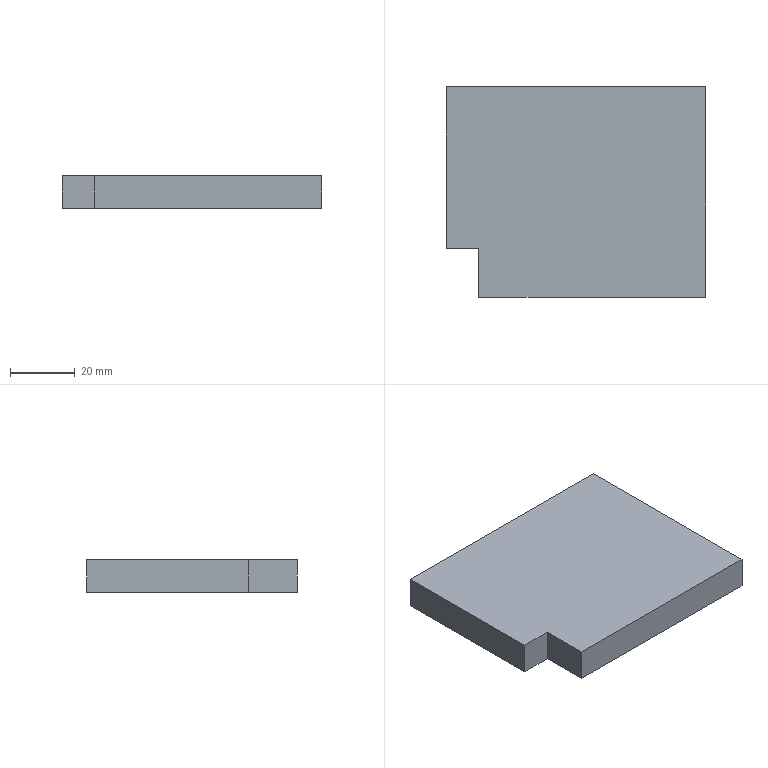Part | NX | features solid 2 | 1 solid | 8 faces | box 80 x 65 x 10 mm | volume 50500 mm3 | plane 8
STEP:
#1=CARTESIAN_POINT('',(-320.,0.,10.));
#2=VERTEX_POINT('',#1);
#3=CARTESIAN_POINT('',(-320.,0.,0.));
#4=VERTEX_POINT('',#3);
#5=CARTESIAN_POINT('',(-320.,0.,0.));
#6=DIRECTION('',(0.,0.,-1.));
#7=VECTOR('',#6,1000.);
#8=LINE('',#5,#7);
#9=EDGE_CURVE('',#2,#4,#8,.T.);
#10=ORIENTED_EDGE('',*,*,#9,.T.);
#11=CARTESIAN_POINT('',(-320.,-15.,0.));
#12=VERTEX_POINT('',#11);
#13=CARTESIAN_POINT('',(-320.,50.,0.));
#14=DIRECTION('',(0.,1.,0.));
#15=VECTOR('',#14,1000.);
#16=LINE('',#13,#15);
#17=EDGE_CURVE('',#12,#4,#16,.T.);
#18=ORIENTED_EDGE('',*,*,#17,.F.);
#19=CARTESIAN_POINT('',(-320.,-15.,10.));
#20=VERTEX_POINT('',#19);
#21=CARTESIAN_POINT('',(-320.,-15.,0.));
#22=DIRECTION('',(0.,0.,-1.));
#23=VECTOR('',#22,1000.);
#24=LINE('',#21,#23);
#25=EDGE_CURVE('',#20,#12,#24,.T.);
#26=ORIENTED_EDGE('',*,*,#25,.F.);
#27=CARTESIAN_POINT('',(-320.,50.,10.));
#28=DIRECTION('',(0.,1.,0.));
#29=VECTOR('',#28,1000.);
#30=LINE('',#27,#29);
#31=EDGE_CURVE('',#20,#2,#30,.T.);
#32=ORIENTED_EDGE('',*,*,#31,.T.);
#33=EDGE_LOOP('',(#10,#18,#26,#32));
#34=FACE_BOUND('',#33,.T.);
#35=CARTESIAN_POINT('',(-320.,50.,0.));
#36=DIRECTION('',(1.,0.,0.));
#37=DIRECTION('',(0.,-1.,0.));
#38=AXIS2_PLACEMENT_3D('',#35,#36,#37);
#39=PLANE('',#38);
#40=ADVANCED_FACE('',(#34),#39,.F.);
#41=CARTESIAN_POINT('',(-330.,0.,10.));
#42=VERTEX_POINT('',#41);
#43=CARTESIAN_POINT('',(-330.,0.,0.));
#44=VERTEX_POINT('',#43);
#45=CARTESIAN_POINT('',(-330.,0.,0.));
#46=DIRECTION('',(0.,0.,-1.));
#47=VECTOR('',#46,1000.);
#48=LINE('',#45,#47);
#49=EDGE_CURVE('',#42,#44,#48,.T.);
#50=ORIENTED_EDGE('',*,*,#49,.T.);
#51=CARTESIAN_POINT('',(-330.,0.,0.));
#52=DIRECTION('',(-1.,0.,0.));
#53=VECTOR('',#52,1000.);
#54=LINE('',#51,#53);
#55=EDGE_CURVE('',#4,#44,#54,.T.);
#56=ORIENTED_EDGE('',*,*,#55,.F.);
#57=ORIENTED_EDGE('',*,*,#9,.F.);
#58=CARTESIAN_POINT('',(-330.,0.,10.));
#59=DIRECTION('',(-1.,0.,0.));
#60=VECTOR('',#59,1000.);
#61=LINE('',#58,#60);
#62=EDGE_CURVE('',#2,#42,#61,.T.);
#63=ORIENTED_EDGE('',*,*,#62,.T.);
#64=EDGE_LOOP('',(#50,#56,#57,#63));
#65=FACE_BOUND('',#64,.T.);
#66=CARTESIAN_POINT('',(-330.,0.,0.));
#67=DIRECTION('',(0.,1.,0.));
#68=DIRECTION('',(1.,0.,0.));
#69=AXIS2_PLACEMENT_3D('',#66,#67,#68);
#70=PLANE('',#69);
#71=ADVANCED_FACE('',(#65),#70,.F.);
#72=CARTESIAN_POINT('',(-250.,-15.,0.));
#73=VERTEX_POINT('',#72);
#74=CARTESIAN_POINT('',(-250.,50.,0.));
#75=VERTEX_POINT('',#74);
#76=CARTESIAN_POINT('',(-250.,-20.,0.));
#77=DIRECTION('',(0.,1.,0.));
#78=VECTOR('',#77,1000.);
#79=LINE('',#76,#78);
#80=EDGE_CURVE('',#73,#75,#79,.T.);
#81=ORIENTED_EDGE('',*,*,#80,.T.);
#82=CARTESIAN_POINT('',(-250.,50.,10.));
#83=VERTEX_POINT('',#82);
#84=CARTESIAN_POINT('',(-250.,50.,10.));
#85=DIRECTION('',(0.,0.,-1.));
#86=VECTOR('',#85,1000.);
#87=LINE('',#84,#86);
#88=EDGE_CURVE('',#83,#75,#87,.T.);
#89=ORIENTED_EDGE('',*,*,#88,.F.);
#90=CARTESIAN_POINT('',(-250.,-15.,10.));
#91=VERTEX_POINT('',#90);
#92=CARTESIAN_POINT('',(-250.,-20.,10.));
#93=DIRECTION('',(0.,-1.,0.));
#94=VECTOR('',#93,1000.);
#95=LINE('',#92,#94);
#96=EDGE_CURVE('',#83,#91,#95,.T.);
#97=ORIENTED_EDGE('',*,*,#96,.T.);
#98=CARTESIAN_POINT('',(-250.,-15.,10.));
#99=DIRECTION('',(0.,0.,-1.));
#100=VECTOR('',#99,1000.);
#101=LINE('',#98,#100);
#102=EDGE_CURVE('',#91,#73,#101,.T.);
#103=ORIENTED_EDGE('',*,*,#102,.T.);
#104=EDGE_LOOP('',(#81,#89,#97,#103));
#105=FACE_BOUND('',#104,.T.);
#106=CARTESIAN_POINT('',(-250.,-20.,10.));
#107=DIRECTION('',(-1.,0.,0.));
#108=DIRECTION('',(0.,0.,1.));
#109=AXIS2_PLACEMENT_3D('',#106,#107,#108);
#110=PLANE('',#109);
#111=ADVANCED_FACE('',(#105),#110,.F.);
#112=ORIENTED_EDGE('',*,*,#17,.T.);
#113=ORIENTED_EDGE('',*,*,#55,.T.);
#114=CARTESIAN_POINT('',(-330.,50.,0.));
#115=VERTEX_POINT('',#114);
#116=CARTESIAN_POINT('',(-330.,50.,0.));
#117=DIRECTION('',(0.,1.,0.));
#118=VECTOR('',#117,1000.);
#119=LINE('',#116,#118);
#120=EDGE_CURVE('',#44,#115,#119,.T.);
#121=ORIENTED_EDGE('',*,*,#120,.T.);
#122=CARTESIAN_POINT('',(-330.,50.,0.));
#123=DIRECTION('',(-1.,0.,0.));
#124=VECTOR('',#123,1000.);
#125=LINE('',#122,#124);
#126=EDGE_CURVE('',#75,#115,#125,.T.);
#127=ORIENTED_EDGE('',*,*,#126,.F.);
#128=ORIENTED_EDGE('',*,*,#80,.F.);
#129=CARTESIAN_POINT('',(-330.,-15.,0.));
#130=DIRECTION('',(-1.,0.,0.));
#131=VECTOR('',#130,1000.);
#132=LINE('',#129,#131);
#133=EDGE_CURVE('',#73,#12,#132,.T.);
#134=ORIENTED_EDGE('',*,*,#133,.T.);
#135=EDGE_LOOP('',(#112,#113,#121,#127,#128,#134));
#136=FACE_BOUND('',#135,.T.);
#137=CARTESIAN_POINT('',(-330.,50.,0.));
#138=DIRECTION('',(0.,0.,1.));
#139=DIRECTION('',(0.,-1.,0.));
#140=AXIS2_PLACEMENT_3D('',#137,#138,#139);
#141=PLANE('',#140);
#142=ADVANCED_FACE('',(#136),#141,.F.);
#143=ORIENTED_EDGE('',*,*,#88,.T.);
#144=ORIENTED_EDGE('',*,*,#126,.T.);
#145=CARTESIAN_POINT('',(-330.,50.,10.));
#146=VERTEX_POINT('',#145);
#147=CARTESIAN_POINT('',(-330.,50.,10.));
#148=DIRECTION('',(0.,0.,1.));
#149=VECTOR('',#148,1000.);
#150=LINE('',#147,#149);
#151=EDGE_CURVE('',#115,#146,#150,.T.);
#152=ORIENTED_EDGE('',*,*,#151,.T.);
#153=CARTESIAN_POINT('',(-330.,50.,10.));
#154=DIRECTION('',(1.,0.,0.));
#155=VECTOR('',#154,1000.);
#156=LINE('',#153,#155);
#157=EDGE_CURVE('',#146,#83,#156,.T.);
#158=ORIENTED_EDGE('',*,*,#157,.T.);
#159=EDGE_LOOP('',(#143,#144,#152,#158));
#160=FACE_BOUND('',#159,.T.);
#161=CARTESIAN_POINT('',(-330.,50.,10.));
#162=DIRECTION('',(0.,1.,0.));
#163=DIRECTION('',(0.,0.,-1.));
#164=AXIS2_PLACEMENT_3D('',#161,#162,#163);
#165=PLANE('',#164);
#166=ADVANCED_FACE('',(#160),#165,.T.);
#167=CARTESIAN_POINT('',(-330.,-20.,10.));
#168=DIRECTION('',(0.,-1.,0.));
#169=VECTOR('',#168,1000.);
#170=LINE('',#167,#169);
#171=EDGE_CURVE('',#146,#42,#170,.T.);
#172=ORIENTED_EDGE('',*,*,#171,.T.);
#173=ORIENTED_EDGE('',*,*,#62,.F.);
#174=ORIENTED_EDGE('',*,*,#31,.F.);
#175=CARTESIAN_POINT('',(-330.,-15.,10.));
#176=DIRECTION('',(1.,0.,0.));
#177=VECTOR('',#176,1000.);
#178=LINE('',#175,#177);
#179=EDGE_CURVE('',#20,#91,#178,.T.);
#180=ORIENTED_EDGE('',*,*,#179,.T.);
#181=ORIENTED_EDGE('',*,*,#96,.F.);
#182=ORIENTED_EDGE('',*,*,#157,.F.);
#183=EDGE_LOOP('',(#172,#173,#174,#180,#181,#182));
#184=FACE_BOUND('',#183,.T.);
#185=CARTESIAN_POINT('',(-330.,-20.,10.));
#186=DIRECTION('',(0.,0.,-1.));
#187=DIRECTION('',(-1.,0.,0.));
#188=AXIS2_PLACEMENT_3D('',#185,#186,#187);
#189=PLANE('',#188);
#190=ADVANCED_FACE('',(#184),#189,.F.);
#191=ORIENTED_EDGE('',*,*,#179,.F.);
#192=ORIENTED_EDGE('',*,*,#25,.T.);
#193=ORIENTED_EDGE('',*,*,#133,.F.);
#194=ORIENTED_EDGE('',*,*,#102,.F.);
#195=EDGE_LOOP('',(#191,#192,#193,#194));
#196=FACE_BOUND('',#195,.T.);
#197=CARTESIAN_POINT('',(-330.,-15.,10.));
#198=DIRECTION('',(0.,1.,0.));
#199=DIRECTION('',(0.,0.,-1.));
#200=AXIS2_PLACEMENT_3D('',#197,#198,#199);
#201=PLANE('',#200);
#202=ADVANCED_FACE('',(#196),#201,.F.);
#203=ORIENTED_EDGE('',*,*,#120,.F.);
#204=ORIENTED_EDGE('',*,*,#49,.F.);
#205=ORIENTED_EDGE('',*,*,#171,.F.);
#206=ORIENTED_EDGE('',*,*,#151,.F.);
#207=EDGE_LOOP('',(#203,#204,#205,#206));
#208=FACE_BOUND('',#207,.T.);
#209=CARTESIAN_POINT('',(-330.,-20.,10.));
#210=DIRECTION('',(1.,0.,0.));
#211=DIRECTION('',(0.,-1.,0.));
#212=AXIS2_PLACEMENT_3D('',#209,#210,#211);
#213=PLANE('',#212);
#214=ADVANCED_FACE('',(#208),#213,.F.);
#215=CLOSED_SHELL('',(#40,#71,#111,#142,#166,#190,#202,#214));
#216=MANIFOLD_SOLID_BREP('',#215);
#217=(LENGTH_UNIT()NAMED_UNIT(*)SI_UNIT(.MILLI.,.METRE.));
#218=UNCERTAINTY_MEASURE_WITH_UNIT(LENGTH_MEASURE(0.00001),#217,'','');
#219=(NAMED_UNIT(*)PLANE_ANGLE_UNIT()SI_UNIT($,.RADIAN.));
#220=(NAMED_UNIT(*)SI_UNIT($,.STERADIAN.)SOLID_ANGLE_UNIT());
#221=(GEOMETRIC_REPRESENTATION_CONTEXT(3)GLOBAL_UNCERTAINTY_ASSIGNED_CONTEXT((#218))GLOBAL_UNIT_ASSIGNED_CONTEXT((#217,#219,#220))REPRESENTATION_CONTEXT('',''));
#222=ADVANCED_BREP_SHAPE_REPRESENTATION('',(#216),#221);